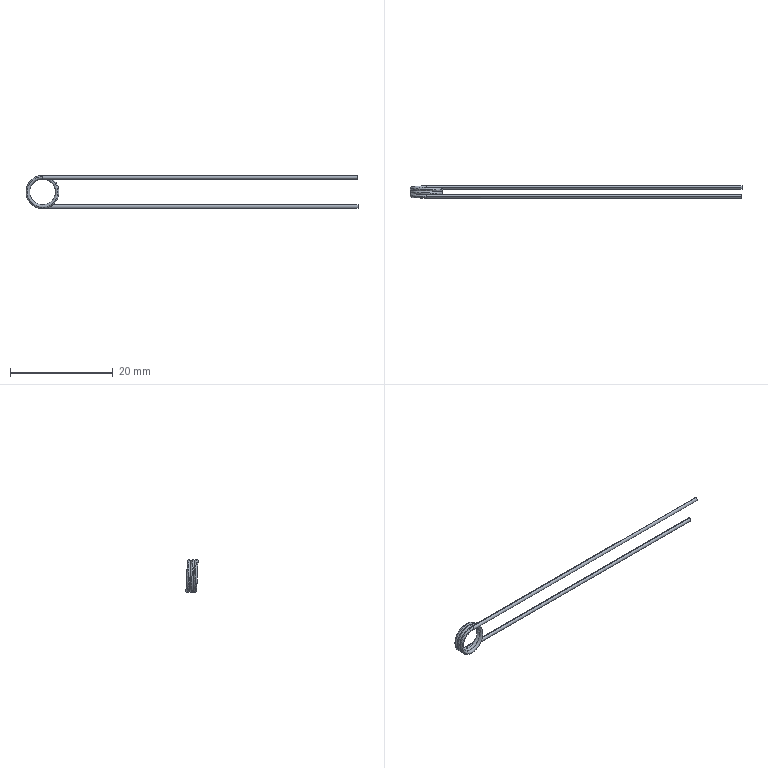Part | SolidWorks | features MoveFace 2, CompositeCurve 1, Helix 1, Sweep 1 | 1 solid | 9 faces | box 64.55 x 2.45 x 6.4 mm | volume 63.849 mm3 | cylinder 4 | spline 3 | plane 2 | commonest cylinder face diameters 0.7 x4
STEP:
#1=CARTESIAN_POINT('',(61.35,1.75,-3.2));
#2=VERTEX_POINT('',#1);
#3=CARTESIAN_POINT('',(61.35,1.75,-2.5));
#4=VERTEX_POINT('',#3);
#5=CARTESIAN_POINT('',(61.35,1.75,-2.85));
#6=DIRECTION('',(1.,0.,0.));
#7=DIRECTION('',(0.,0.00009155,-1.));
#8=AXIS2_PLACEMENT_3D('',#5,#6,#7);
#9=CIRCLE('',#8,0.35);
#10=EDGE_CURVE('',#2,#4,#9,.T.);
#11=ORIENTED_EDGE('',*,*,#10,.F.);
#12=CARTESIAN_POINT('',(-0.000000536,1.75,-3.2));
#13=VERTEX_POINT('',#12);
#14=CARTESIAN_POINT('',(12.85,1.75,-3.2));
#15=DIRECTION('',(-1.,0.,0.));
#16=VECTOR('',#15,1000.);
#17=LINE('',#14,#16);
#18=EDGE_CURVE('',#2,#13,#17,.T.);
#19=ORIENTED_EDGE('',*,*,#18,.T.);
#20=CARTESIAN_POINT('',(-0.006305,2.074,-2.979));
#21=VERTEX_POINT('',#20);
#22=CARTESIAN_POINT('',(0.,1.75,-2.85));
#23=DIRECTION('',(1.,0.,0.));
#24=DIRECTION('',(0.,0.00009155,-1.));
#25=AXIS2_PLACEMENT_3D('',#22,#23,#24);
#26=CIRCLE('',#25,0.35);
#27=EDGE_CURVE('',#13,#21,#26,.T.);
#28=ORIENTED_EDGE('',*,*,#27,.T.);
#29=CARTESIAN_POINT('',(0.,1.75,-2.5));
#30=VERTEX_POINT('',#29);
#31=CARTESIAN_POINT('',(0.,1.75,-2.85));
#32=DIRECTION('',(1.,0.,0.));
#33=DIRECTION('',(0.,0.00009155,-1.));
#34=AXIS2_PLACEMENT_3D('',#31,#32,#33);
#35=CIRCLE('',#34,0.35);
#36=EDGE_CURVE('',#21,#30,#35,.T.);
#37=ORIENTED_EDGE('',*,*,#36,.T.);
#38=CARTESIAN_POINT('',(12.85,1.75,-2.5));
#39=DIRECTION('',(-1.,0.,0.));
#40=VECTOR('',#39,1000.);
#41=LINE('',#38,#40);
#42=EDGE_CURVE('',#4,#30,#41,.T.);
#43=ORIENTED_EDGE('',*,*,#42,.F.);
#44=EDGE_LOOP('',(#11,#19,#28,#37,#43));
#45=FACE_OUTER_BOUND('',#44,.T.);
#46=CARTESIAN_POINT('',(12.85,1.75,-2.85));
#47=DIRECTION('',(-1.,0.,0.));
#48=DIRECTION('',(0.,0.,1.));
#49=AXIS2_PLACEMENT_3D('',#46,#47,#48);
#50=CYLINDRICAL_SURFACE('',#49,0.35);
#51=ADVANCED_FACE('',(#45),#50,.T.);
#52=CARTESIAN_POINT('',(0.006305,0.3239,2.979));
#53=VERTEX_POINT('',#52);
#54=CARTESIAN_POINT('',(0.,0.,3.2));
#55=VERTEX_POINT('',#54);
#56=CARTESIAN_POINT('',(0.006305,0.3239,2.979));
#57=CARTESIAN_POINT('',(0.01048,0.2681,3.104));
#58=CARTESIAN_POINT('',(0.005425,0.1388,3.2));
#59=CARTESIAN_POINT('',(0.,0.,3.2));
#60=B_SPLINE_CURVE_WITH_KNOTS('',3,(#56,#57,#58,#59),.UNSPECIFIED.,.F.,.F.,(4,4),(0.00002721,0.1895),.UNSPECIFIED.);
#61=EDGE_CURVE('',#53,#55,#60,.T.);
#62=ORIENTED_EDGE('',*,*,#61,.T.);
#63=CARTESIAN_POINT('',(61.35,0.,3.2));
#64=VERTEX_POINT('',#63);
#65=CARTESIAN_POINT('',(0.,0.,3.2));
#66=DIRECTION('',(1.,0.,0.));
#67=VECTOR('',#66,1000.);
#68=LINE('',#65,#67);
#69=EDGE_CURVE('',#55,#64,#68,.T.);
#70=ORIENTED_EDGE('',*,*,#69,.T.);
#71=CARTESIAN_POINT('',(61.35,0.,2.5));
#72=VERTEX_POINT('',#71);
#73=CARTESIAN_POINT('',(61.35,0.,2.85));
#74=DIRECTION('',(-1.,0.,0.));
#75=DIRECTION('',(0.,0.,1.));
#76=AXIS2_PLACEMENT_3D('',#73,#74,#75);
#77=CIRCLE('',#76,0.35);
#78=EDGE_CURVE('',#64,#72,#77,.T.);
#79=ORIENTED_EDGE('',*,*,#78,.T.);
#80=CARTESIAN_POINT('',(0.,0.,2.5));
#81=VERTEX_POINT('',#80);
#82=CARTESIAN_POINT('',(0.,0.,2.5));
#83=DIRECTION('',(1.,0.,0.));
#84=VECTOR('',#83,1000.);
#85=LINE('',#82,#84);
#86=EDGE_CURVE('',#81,#72,#85,.T.);
#87=ORIENTED_EDGE('',*,*,#86,.F.);
#88=CARTESIAN_POINT('',(0.,0.,2.85));
#89=DIRECTION('',(-1.,0.,0.));
#90=DIRECTION('',(0.,0.,1.));
#91=AXIS2_PLACEMENT_3D('',#88,#89,#90);
#92=CIRCLE('',#91,0.35);
#93=EDGE_CURVE('',#53,#81,#92,.T.);
#94=ORIENTED_EDGE('',*,*,#93,.F.);
#95=EDGE_LOOP('',(#62,#70,#79,#87,#94));
#96=FACE_OUTER_BOUND('',#95,.T.);
#97=CARTESIAN_POINT('',(0.,0.,2.85));
#98=DIRECTION('',(1.,0.,0.));
#99=DIRECTION('',(0.,0.,-1.));
#100=AXIS2_PLACEMENT_3D('',#97,#98,#99);
#101=CYLINDRICAL_SURFACE('',#100,0.35);
#102=ADVANCED_FACE('',(#96),#101,.T.);
#103=ORIENTED_EDGE('',*,*,#18,.F.);
#104=CARTESIAN_POINT('',(61.35,1.75,-2.85));
#105=DIRECTION('',(1.,0.,0.));
#106=DIRECTION('',(0.,0.00009155,-1.));
#107=AXIS2_PLACEMENT_3D('',#104,#105,#106);
#108=CIRCLE('',#107,0.35);
#109=EDGE_CURVE('',#4,#2,#108,.T.);
#110=ORIENTED_EDGE('',*,*,#109,.F.);
#111=ORIENTED_EDGE('',*,*,#42,.T.);
#112=CARTESIAN_POINT('',(0.006304,1.426,-2.979));
#113=VERTEX_POINT('',#112);
#114=CARTESIAN_POINT('',(0.,1.75,-2.85));
#115=DIRECTION('',(1.,0.,0.));
#116=DIRECTION('',(0.,0.00009155,-1.));
#117=AXIS2_PLACEMENT_3D('',#114,#115,#116);
#118=CIRCLE('',#117,0.35);
#119=EDGE_CURVE('',#30,#113,#118,.T.);
#120=ORIENTED_EDGE('',*,*,#119,.T.);
#121=CARTESIAN_POINT('',(0.,1.75,-2.85));
#122=DIRECTION('',(1.,0.,0.));
#123=DIRECTION('',(0.,0.00009155,-1.));
#124=AXIS2_PLACEMENT_3D('',#121,#122,#123);
#125=CIRCLE('',#124,0.35);
#126=EDGE_CURVE('',#113,#13,#125,.T.);
#127=ORIENTED_EDGE('',*,*,#126,.T.);
#128=EDGE_LOOP('',(#103,#110,#111,#120,#127));
#129=FACE_OUTER_BOUND('',#128,.T.);
#130=CARTESIAN_POINT('',(12.85,1.75,-2.85));
#131=DIRECTION('',(-1.,0.,0.));
#132=DIRECTION('',(0.,0.,1.));
#133=AXIS2_PLACEMENT_3D('',#130,#131,#132);
#134=CYLINDRICAL_SURFACE('',#133,0.35);
#135=ADVANCED_FACE('',(#129),#134,.T.);
#136=ORIENTED_EDGE('',*,*,#36,.F.);
#137=CARTESIAN_POINT('',(0.006305,0.3239,2.979));
#138=CARTESIAN_POINT('',(-0.7712,0.3519,2.981));
#139=CARTESIAN_POINT('',(-1.545,0.381,2.663));
#140=CARTESIAN_POINT('',(-2.649,0.4392,1.566));
#141=CARTESIAN_POINT('',(-2.975,0.4683,0.7939));
#142=CARTESIAN_POINT('',(-2.98,0.5195,-0.5733));
#143=CARTESIAN_POINT('',(-2.806,0.5413,-1.156));
#144=CARTESIAN_POINT('',(-2.162,0.585,-2.13));
#145=CARTESIAN_POINT('',(-1.69,0.6069,-2.521));
#146=CARTESIAN_POINT('',(-0.4324,0.658,-3.048));
#147=CARTESIAN_POINT('',(0.405,0.6871,-3.052));
#148=CARTESIAN_POINT('',(1.67,0.7383,-2.534));
#149=CARTESIAN_POINT('',(2.142,0.7601,-2.15));
#150=CARTESIAN_POINT('',(2.795,0.8037,-1.182));
#151=CARTESIAN_POINT('',(2.976,0.8257,-0.5972));
#152=CARTESIAN_POINT('',(2.981,0.8768,0.7668));
#153=CARTESIAN_POINT('',(2.665,0.9058,1.542));
#154=CARTESIAN_POINT('',(1.702,0.957,2.513));
#155=CARTESIAN_POINT('',(1.167,0.9788,2.801));
#156=CARTESIAN_POINT('',(0.02248,1.022,3.035));
#157=CARTESIAN_POINT('',(-0.587,1.044,2.978));
#158=CARTESIAN_POINT('',(-1.849,1.096,2.461));
#159=CARTESIAN_POINT('',(-2.445,1.125,1.872));
#160=CARTESIAN_POINT('',(-2.973,1.176,0.6109));
#161=CARTESIAN_POINT('',(-3.035,1.198,0.005944));
#162=CARTESIAN_POINT('',(-2.812,1.241,-1.14));
#163=CARTESIAN_POINT('',(-2.526,1.263,-1.682));
#164=CARTESIAN_POINT('',(-1.566,1.314,-2.65));
#165=CARTESIAN_POINT('',(-0.7938,1.343,-2.975));
#166=CARTESIAN_POINT('',(0.5733,1.395,-2.98));
#167=CARTESIAN_POINT('',(1.156,1.416,-2.806));
#168=CARTESIAN_POINT('',(2.13,1.46,-2.162));
#169=CARTESIAN_POINT('',(2.521,1.482,-1.69));
#170=CARTESIAN_POINT('',(3.048,1.533,-0.4324));
#171=CARTESIAN_POINT('',(3.052,1.562,0.405));
#172=CARTESIAN_POINT('',(2.534,1.613,1.67));
#173=CARTESIAN_POINT('',(2.15,1.635,2.142));
#174=CARTESIAN_POINT('',(1.182,1.679,2.795));
#175=CARTESIAN_POINT('',(0.5972,1.701,2.976));
#176=CARTESIAN_POINT('',(-0.7668,1.752,2.981));
#177=CARTESIAN_POINT('',(-1.542,1.781,2.665));
#178=CARTESIAN_POINT('',(-2.513,1.832,1.702));
#179=CARTESIAN_POINT('',(-2.801,1.854,1.167));
#180=CARTESIAN_POINT('',(-3.034,1.897,0.0225));
#181=CARTESIAN_POINT('',(-2.978,1.919,-0.587));
#182=CARTESIAN_POINT('',(-2.46,1.971,-1.85));
#183=CARTESIAN_POINT('',(-1.872,2.,-2.445));
#184=CARTESIAN_POINT('',(-0.7917,2.043,-2.897));
#185=CARTESIAN_POINT('',(-0.4042,2.058,-2.976));
#186=CARTESIAN_POINT('',(-0.006305,2.074,-2.979));
#187=B_SPLINE_CURVE_WITH_KNOTS('',3,(#137,#138,#139,#140,#141,#142,#143,#144,#145,#146,#147,#148,#149,#150,#151,#152,#153,#154,#155,#156,#157,#158,#159,#160,#161,#162,#163,#164,#165,#166,#167,#168,#169,#170,#171,#172,#173,#174,#175,#176,#177,#178,#179,#180,#181,#182,#183,#184,#185,#186),.UNSPECIFIED.,.F.,.F.,(4,2,2,2,2,2,2,2,2,2,2,2,2,2,2,2,2,2,2,2,2,2,2,2,4),(0.,0.04998,0.09999,0.1375,0.175,0.225,0.2625,0.3,0.35,0.3875,0.425,0.475,0.5125,0.55,0.6,0.6375,0.675,0.725,0.7625,0.8,0.85,0.8875,0.925,0.975,1.),.UNSPECIFIED.);
#188=EDGE_CURVE('',#53,#21,#187,.T.);
#189=ORIENTED_EDGE('',*,*,#188,.F.);
#190=ORIENTED_EDGE('',*,*,#93,.T.);
#191=CARTESIAN_POINT('',(-0.006304,-0.3239,2.979));
#192=VERTEX_POINT('',#191);
#193=CARTESIAN_POINT('',(0.,0.,2.85));
#194=DIRECTION('',(-1.,0.,0.));
#195=DIRECTION('',(0.,0.,1.));
#196=AXIS2_PLACEMENT_3D('',#193,#194,#195);
#197=CIRCLE('',#196,0.35);
#198=EDGE_CURVE('',#81,#192,#197,.T.);
#199=ORIENTED_EDGE('',*,*,#198,.T.);
#200=CARTESIAN_POINT('',(0.006304,1.426,-2.979));
#201=CARTESIAN_POINT('',(-0.379,1.413,-2.98));
#202=CARTESIAN_POINT('',(-0.7673,1.398,-2.904));
#203=CARTESIAN_POINT('',(-1.851,1.354,-2.461));
#204=CARTESIAN_POINT('',(-2.445,1.325,-1.871));
#205=CARTESIAN_POINT('',(-2.973,1.274,-0.6122));
#206=CARTESIAN_POINT('',(-3.035,1.252,-0.003211));
#207=CARTESIAN_POINT('',(-2.811,1.209,1.143));
#208=CARTESIAN_POINT('',(-2.527,1.187,1.681));
#209=CARTESIAN_POINT('',(-1.565,1.136,2.652));
#210=CARTESIAN_POINT('',(-0.792,1.107,2.975));
#211=CARTESIAN_POINT('',(0.572,1.056,2.981));
#212=CARTESIAN_POINT('',(1.158,1.034,2.805));
#213=CARTESIAN_POINT('',(2.132,0.99,2.16));
#214=CARTESIAN_POINT('',(2.52,0.9682,1.692));
#215=CARTESIAN_POINT('',(3.049,0.917,0.4308));
#216=CARTESIAN_POINT('',(3.052,0.8879,-0.4067));
#217=CARTESIAN_POINT('',(2.535,0.8368,-1.669));
#218=CARTESIAN_POINT('',(2.148,0.8149,-2.144));
#219=CARTESIAN_POINT('',(1.18,0.7712,-2.796));
#220=CARTESIAN_POINT('',(0.5985,0.7494,-2.976));
#221=CARTESIAN_POINT('',(-0.7686,0.6982,-2.981));
#222=CARTESIAN_POINT('',(-1.544,0.6692,-2.664));
#223=CARTESIAN_POINT('',(-2.512,0.6181,-1.703));
#224=CARTESIAN_POINT('',(-2.802,0.5961,-1.164));
#225=CARTESIAN_POINT('',(-3.035,0.5525,-0.01977));
#226=CARTESIAN_POINT('',(-2.978,0.5307,0.5858));
#227=CARTESIAN_POINT('',(-2.46,0.4795,1.851));
#228=CARTESIAN_POINT('',(-1.87,0.4504,2.445));
#229=CARTESIAN_POINT('',(-0.6122,0.3993,2.973));
#230=CARTESIAN_POINT('',(-0.003226,0.3774,3.035));
#231=CARTESIAN_POINT('',(1.143,0.3337,2.811));
#232=CARTESIAN_POINT('',(1.681,0.3119,2.527));
#233=CARTESIAN_POINT('',(2.652,0.2607,1.565));
#234=CARTESIAN_POINT('',(2.975,0.2317,0.792));
#235=CARTESIAN_POINT('',(2.981,0.1806,-0.572));
#236=CARTESIAN_POINT('',(2.805,0.1586,-1.158));
#237=CARTESIAN_POINT('',(2.16,0.115,-2.132));
#238=CARTESIAN_POINT('',(1.692,0.09317,-2.52));
#239=CARTESIAN_POINT('',(0.4308,0.04196,-3.049));
#240=CARTESIAN_POINT('',(-0.4067,0.01292,-3.052));
#241=CARTESIAN_POINT('',(-1.669,-0.03818,-2.535));
#242=CARTESIAN_POINT('',(-2.144,-0.06013,-2.148));
#243=CARTESIAN_POINT('',(-2.796,-0.1038,-1.18));
#244=CARTESIAN_POINT('',(-2.976,-0.1256,-0.5985));
#245=CARTESIAN_POINT('',(-2.981,-0.1768,0.7687));
#246=CARTESIAN_POINT('',(-2.663,-0.2059,1.544));
#247=CARTESIAN_POINT('',(-1.567,-0.2642,2.65));
#248=CARTESIAN_POINT('',(-0.7966,-0.2932,2.975));
#249=CARTESIAN_POINT('',(-0.006304,-0.3239,2.979));
#250=B_SPLINE_CURVE_WITH_KNOTS('',3,(#200,#201,#202,#203,#204,#205,#206,#207,#208,#209,#210,#211,#212,#213,#214,#215,#216,#217,#218,#219,#220,#221,#222,#223,#224,#225,#226,#227,#228,#229,#230,#231,#232,#233,#234,#235,#236,#237,#238,#239,#240,#241,#242,#243,#244,#245,#246,#247,#248,#249),.UNSPECIFIED.,.F.,.F.,(4,2,2,2,2,2,2,2,2,2,2,2,2,2,2,2,2,2,2,2,2,2,2,2,4),(0.,0.02496,0.07501,0.1125,0.15,0.2,0.2375,0.275,0.325,0.3625,0.4,0.45,0.4875,0.525,0.575,0.6125,0.65,0.7,0.7375,0.775,0.825,0.8625,0.9,0.95,1.),.UNSPECIFIED.);
#251=EDGE_CURVE('',#113,#192,#250,.T.);
#252=ORIENTED_EDGE('',*,*,#251,.F.);
#253=ORIENTED_EDGE('',*,*,#119,.F.);
#254=EDGE_LOOP('',(#136,#189,#190,#199,#252,#253));
#255=FACE_OUTER_BOUND('',#254,.T.);
#256=CARTESIAN_POINT('',(-0.01261,2.073,-2.978));
#257=CARTESIAN_POINT('',(-0.9931,2.036,-2.974));
#258=CARTESIAN_POINT('',(-1.942,2.,-2.452));
#259=CARTESIAN_POINT('',(-3.022,1.927,-0.8338));
#260=CARTESIAN_POINT('',(-3.123,1.89,0.2539));
#261=CARTESIAN_POINT('',(-2.369,1.817,2.048));
#262=CARTESIAN_POINT('',(-1.523,1.781,2.732));
#263=CARTESIAN_POINT('',(0.3864,1.708,3.111));
#264=CARTESIAN_POINT('',(1.43,1.671,2.788));
#265=CARTESIAN_POINT('',(2.798,1.599,1.405));
#266=CARTESIAN_POINT('',(3.107,1.562,0.3615));
#267=CARTESIAN_POINT('',(2.726,1.489,-1.547));
#268=CARTESIAN_POINT('',(2.029,1.453,-2.388));
#269=CARTESIAN_POINT('',(0.2273,1.38,-3.123));
#270=CARTESIAN_POINT('',(-0.8551,1.343,-3.009));
#271=CARTESIAN_POINT('',(-2.473,1.271,-1.927));
#272=CARTESIAN_POINT('',(-2.982,1.234,-0.9604));
#273=CARTESIAN_POINT('',(-2.972,1.161,0.9852));
#274=CARTESIAN_POINT('',(-2.453,1.125,1.942));
#275=CARTESIAN_POINT('',(-0.8335,1.052,3.022));
#276=CARTESIAN_POINT('',(0.2539,1.015,3.123));
#277=CARTESIAN_POINT('',(2.048,0.9425,2.369));
#278=CARTESIAN_POINT('',(2.732,0.9059,1.523));
#279=CARTESIAN_POINT('',(3.111,0.8331,-0.3864));
#280=CARTESIAN_POINT('',(2.788,0.7965,-1.43));
#281=CARTESIAN_POINT('',(1.405,0.7237,-2.798));
#282=CARTESIAN_POINT('',(0.3615,0.6872,-3.107));
#283=CARTESIAN_POINT('',(-1.547,0.6143,-2.726));
#284=CARTESIAN_POINT('',(-2.388,0.5777,-2.029));
#285=CARTESIAN_POINT('',(-3.123,0.505,-0.2273));
#286=CARTESIAN_POINT('',(-3.009,0.4684,0.8554));
#287=CARTESIAN_POINT('',(-1.927,0.3956,2.473));
#288=CARTESIAN_POINT('',(-0.9676,0.3593,2.982));
#289=CARTESIAN_POINT('',(0.01261,0.3226,2.978));
#290=CARTESIAN_POINT('',(-0.0161,2.162,-2.771));
#291=CARTESIAN_POINT('',(-0.9269,2.125,-2.766));
#292=CARTESIAN_POINT('',(-1.811,2.089,-2.279));
#293=CARTESIAN_POINT('',(-2.813,2.016,-0.7712));
#294=CARTESIAN_POINT('',(-2.906,1.979,0.2409));
#295=CARTESIAN_POINT('',(-2.201,1.907,1.909));
#296=CARTESIAN_POINT('',(-1.413,1.87,2.545));
#297=CARTESIAN_POINT('',(0.3644,1.797,2.894));
#298=CARTESIAN_POINT('',(1.334,1.761,2.592));
#299=CARTESIAN_POINT('',(2.606,1.688,1.303));
#300=CARTESIAN_POINT('',(2.892,1.651,0.3318));
#301=CARTESIAN_POINT('',(2.535,1.579,-1.444));
#302=CARTESIAN_POINT('',(1.884,1.542,-2.225));
#303=CARTESIAN_POINT('',(0.2064,1.469,-2.907));
#304=CARTESIAN_POINT('',(-0.8001,1.433,-2.799));
#305=CARTESIAN_POINT('',(-2.304,1.36,-1.789));
#306=CARTESIAN_POINT('',(-2.777,1.323,-0.8894));
#307=CARTESIAN_POINT('',(-2.764,1.25,0.9216));
#308=CARTESIAN_POINT('',(-2.279,1.214,1.81));
#309=CARTESIAN_POINT('',(-0.771,1.141,2.814));
#310=CARTESIAN_POINT('',(0.2409,1.104,2.906));
#311=CARTESIAN_POINT('',(1.909,1.032,2.201));
#312=CARTESIAN_POINT('',(2.545,0.9951,1.413));
#313=CARTESIAN_POINT('',(2.894,0.9223,-0.3644));
#314=CARTESIAN_POINT('',(2.592,0.8857,-1.334));
#315=CARTESIAN_POINT('',(1.303,0.8129,-2.606));
#316=CARTESIAN_POINT('',(0.3318,0.7764,-2.892));
#317=CARTESIAN_POINT('',(-1.444,0.7035,-2.535));
#318=CARTESIAN_POINT('',(-2.225,0.667,-1.884));
#319=CARTESIAN_POINT('',(-2.907,0.5942,-0.2064));
#320=CARTESIAN_POINT('',(-2.798,0.5576,0.8003));
#321=CARTESIAN_POINT('',(-1.789,0.4848,2.304));
#322=CARTESIAN_POINT('',(-0.8958,0.4485,2.776));
#323=CARTESIAN_POINT('',(0.0161,0.4118,2.771));
#324=CARTESIAN_POINT('',(-0.008888,1.977,-2.5));
#325=CARTESIAN_POINT('',(-0.8283,1.941,-2.497));
#326=CARTESIAN_POINT('',(-1.629,1.904,-2.059));
#327=CARTESIAN_POINT('',(-2.536,1.832,-0.7012));
#328=CARTESIAN_POINT('',(-2.622,1.795,0.2114));
#329=CARTESIAN_POINT('',(-1.989,1.722,1.718));
#330=CARTESIAN_POINT('',(-1.28,1.686,2.292));
#331=CARTESIAN_POINT('',(0.3232,1.613,2.612));
#332=CARTESIAN_POINT('',(1.199,1.576,2.341));
#333=CARTESIAN_POINT('',(2.349,1.503,1.18));
#334=CARTESIAN_POINT('',(2.608,1.467,0.3051));
#335=CARTESIAN_POINT('',(2.29,1.394,-1.298));
#336=CARTESIAN_POINT('',(1.704,1.358,-2.003));
#337=CARTESIAN_POINT('',(0.1914,1.285,-2.622));
#338=CARTESIAN_POINT('',(-0.716,1.248,-2.526));
#339=CARTESIAN_POINT('',(-2.075,1.175,-1.618));
#340=CARTESIAN_POINT('',(-2.503,1.139,-0.808));
#341=CARTESIAN_POINT('',(-2.495,1.066,0.8264));
#342=CARTESIAN_POINT('',(-2.06,1.029,1.628));
#343=CARTESIAN_POINT('',(-0.701,0.9565,2.537));
#344=CARTESIAN_POINT('',(0.2114,0.92,2.622));
#345=CARTESIAN_POINT('',(1.718,0.8471,1.989));
#346=CARTESIAN_POINT('',(2.292,0.8107,1.28));
#347=CARTESIAN_POINT('',(2.612,0.7378,-0.3232));
#348=CARTESIAN_POINT('',(2.341,0.7013,-1.199));
#349=CARTESIAN_POINT('',(1.18,0.6284,-2.349));
#350=CARTESIAN_POINT('',(0.3051,0.5919,-2.608));
#351=CARTESIAN_POINT('',(-1.298,0.519,-2.29));
#352=CARTESIAN_POINT('',(-2.003,0.4825,-1.704));
#353=CARTESIAN_POINT('',(-2.622,0.4096,-0.1914));
#354=CARTESIAN_POINT('',(-2.525,0.3732,0.7162));
#355=CARTESIAN_POINT('',(-1.619,0.3003,2.075));
#356=CARTESIAN_POINT('',(-0.8134,0.2639,2.503));
#357=CARTESIAN_POINT('',(0.008889,0.2274,2.5));
#358=CARTESIAN_POINT('',(0.008895,1.522,-2.5));
#359=CARTESIAN_POINT('',(-0.8105,1.486,-2.503));
#360=CARTESIAN_POINT('',(-1.614,1.45,-2.071));
#361=CARTESIAN_POINT('',(-2.532,1.377,-0.7193));
#362=CARTESIAN_POINT('',(-2.623,1.34,0.1927));
#363=CARTESIAN_POINT('',(-2.001,1.267,1.704));
#364=CARTESIAN_POINT('',(-1.296,1.231,2.283));
#365=CARTESIAN_POINT('',(0.3046,1.158,2.614));
#366=CARTESIAN_POINT('',(1.182,1.121,2.35));
#367=CARTESIAN_POINT('',(2.341,1.048,1.197));
#368=CARTESIAN_POINT('',(2.606,1.012,0.3236));
#369=CARTESIAN_POINT('',(2.299,0.9391,-1.282));
#370=CARTESIAN_POINT('',(1.719,0.9026,-1.991));
#371=CARTESIAN_POINT('',(0.2101,0.8297,-2.62));
#372=CARTESIAN_POINT('',(-0.6981,0.7933,-2.531));
#373=CARTESIAN_POINT('',(-2.064,0.7204,-1.633));
#374=CARTESIAN_POINT('',(-2.497,0.6839,-0.8259));
#375=CARTESIAN_POINT('',(-2.501,0.611,0.8087));
#376=CARTESIAN_POINT('',(-2.071,0.5745,1.614));
#377=CARTESIAN_POINT('',(-0.7191,0.5016,2.532));
#378=CARTESIAN_POINT('',(0.1927,0.4651,2.623));
#379=CARTESIAN_POINT('',(1.704,0.3922,2.001));
#380=CARTESIAN_POINT('',(2.283,0.3558,1.296));
#381=CARTESIAN_POINT('',(2.614,0.2829,-0.3046));
#382=CARTESIAN_POINT('',(2.35,0.2464,-1.182));
#383=CARTESIAN_POINT('',(1.197,0.1735,-2.341));
#384=CARTESIAN_POINT('',(0.3236,0.137,-2.606));
#385=CARTESIAN_POINT('',(-1.282,0.0641,-2.299));
#386=CARTESIAN_POINT('',(-1.991,0.02763,-1.719));
#387=CARTESIAN_POINT('',(-2.62,-0.04528,-0.2101));
#388=CARTESIAN_POINT('',(-2.531,-0.08173,0.6983));
#389=CARTESIAN_POINT('',(-1.633,-0.1546,2.064));
#390=CARTESIAN_POINT('',(-0.8313,-0.191,2.497));
#391=CARTESIAN_POINT('',(-0.008894,-0.2275,2.5));
#392=CARTESIAN_POINT('',(0.0161,1.338,-2.771));
#393=CARTESIAN_POINT('',(-0.8947,1.302,-2.777));
#394=CARTESIAN_POINT('',(-1.785,1.265,-2.3));
#395=CARTESIAN_POINT('',(-2.804,1.192,-0.804));
#396=CARTESIAN_POINT('',(-2.908,1.156,0.2071));
#397=CARTESIAN_POINT('',(-2.223,1.083,1.884));
#398=CARTESIAN_POINT('',(-1.443,1.046,2.528));
#399=CARTESIAN_POINT('',(0.3307,0.9736,2.899));
#400=CARTESIAN_POINT('',(1.304,0.937,2.608));
#401=CARTESIAN_POINT('',(2.591,0.8642,1.333));
#402=CARTESIAN_POINT('',(2.888,0.8277,0.3653));
#403=CARTESIAN_POINT('',(2.552,0.7548,-1.415));
#404=CARTESIAN_POINT('',(1.91,0.7183,-2.203));
#405=CARTESIAN_POINT('',(0.2402,0.6455,-2.904));
#406=CARTESIAN_POINT('',(-0.7677,0.6089,-2.808));
#407=CARTESIAN_POINT('',(-2.284,0.5361,-1.816));
#408=CARTESIAN_POINT('',(-2.766,0.4995,-0.9217));
#409=CARTESIAN_POINT('',(-2.775,0.4267,0.8895));
#410=CARTESIAN_POINT('',(-2.3,0.3902,1.784));
#411=CARTESIAN_POINT('',(-0.8038,0.3173,2.805));
#412=CARTESIAN_POINT('',(0.2071,0.2808,2.908));
#413=CARTESIAN_POINT('',(1.884,0.208,2.223));
#414=CARTESIAN_POINT('',(2.528,0.1714,1.443));
#415=CARTESIAN_POINT('',(2.899,0.09857,-0.3307));
#416=CARTESIAN_POINT('',(2.608,0.06204,-1.304));
#417=CARTESIAN_POINT('',(1.333,-0.01079,-2.591));
#418=CARTESIAN_POINT('',(0.3653,-0.0473,-2.888));
#419=CARTESIAN_POINT('',(-1.415,-0.1202,-2.552));
#420=CARTESIAN_POINT('',(-2.203,-0.1567,-1.91));
#421=CARTESIAN_POINT('',(-2.904,-0.2295,-0.2402));
#422=CARTESIAN_POINT('',(-2.807,-0.2661,0.7679));
#423=CARTESIAN_POINT('',(-1.816,-0.3389,2.283));
#424=CARTESIAN_POINT('',(-0.9282,-0.3752,2.766));
#425=CARTESIAN_POINT('',(-0.0161,-0.4119,2.771));
#426=CARTESIAN_POINT('',(0.01261,1.427,-2.978));
#427=CARTESIAN_POINT('',(-0.9679,1.391,-2.982));
#428=CARTESIAN_POINT('',(-1.922,1.354,-2.469));
#429=CARTESIAN_POINT('',(-3.015,1.282,-0.8595));
#430=CARTESIAN_POINT('',(-3.125,1.245,0.2275));
#431=CARTESIAN_POINT('',(-2.386,1.172,2.028));
#432=CARTESIAN_POINT('',(-1.546,1.136,2.72));
#433=CARTESIAN_POINT('',(0.36,1.063,3.114));
#434=CARTESIAN_POINT('',(1.406,1.026,2.8));
#435=CARTESIAN_POINT('',(2.787,0.9536,1.429));
#436=CARTESIAN_POINT('',(3.104,0.917,0.3878));
#437=CARTESIAN_POINT('',(2.739,0.8442,-1.524));
#438=CARTESIAN_POINT('',(2.049,0.8076,-2.37));
#439=CARTESIAN_POINT('',(0.2537,0.7349,-3.121));
#440=CARTESIAN_POINT('',(-0.8297,0.6983,-3.016));
#441=CARTESIAN_POINT('',(-2.457,0.6254,-1.948));
#442=CARTESIAN_POINT('',(-2.974,0.5889,-0.9857));
#443=CARTESIAN_POINT('',(-2.981,0.5161,0.96));
#444=CARTESIAN_POINT('',(-2.469,0.4795,1.921));
#445=CARTESIAN_POINT('',(-0.8592,0.4067,3.015));
#446=CARTESIAN_POINT('',(0.2275,0.3701,3.125));
#447=CARTESIAN_POINT('',(2.028,0.2974,2.386));
#448=CARTESIAN_POINT('',(2.72,0.2608,1.546));
#449=CARTESIAN_POINT('',(3.114,0.1879,-0.36));
#450=CARTESIAN_POINT('',(2.8,0.1514,-1.406));
#451=CARTESIAN_POINT('',(1.429,0.07861,-2.787));
#452=CARTESIAN_POINT('',(0.3878,0.04204,-3.104));
#453=CARTESIAN_POINT('',(-1.524,-0.03081,-2.739));
#454=CARTESIAN_POINT('',(-2.371,-0.06738,-2.049));
#455=CARTESIAN_POINT('',(-3.121,-0.1401,-0.2537));
#456=CARTESIAN_POINT('',(-3.016,-0.1767,0.83));
#457=CARTESIAN_POINT('',(-1.948,-0.2496,2.456));
#458=CARTESIAN_POINT('',(-0.993,-0.2858,2.974));
#459=CARTESIAN_POINT('',(-0.01261,-0.3225,2.978));
#460=B_SPLINE_SURFACE_WITH_KNOTS('',3,3,((#256,#257,#258,#259,#260,#261,#262,#263,#264,#265,#266,#267,#268,#269,#270,#271,#272,#273,#274,#275,#276,#277,#278,#279,#280,#281,#282,#283,#284,#285,#286,#287,#288,#289),(#290,#291,#292,#293,#294,#295,#296,#297,#298,#299,#300,#301,#302,#303,#304,#305,#306,#307,#308,#309,#310,#311,#312,#313,#314,#315,#316,#317,#318,#319,#320,#321,#322,#323),(#324,#325,#326,#327,#328,#329,#330,#331,#332,#333,#334,#335,#336,#337,#338,#339,#340,#341,#342,#343,#344,#345,#346,#347,#348,#349,#350,#351,#352,#353,#354,#355,#356,#357),(#358,#359,#360,#361,#362,#363,#364,#365,#366,#367,#368,#369,#370,#371,#372,#373,#374,#375,#376,#377,#378,#379,#380,#381,#382,#383,#384,#385,#386,#387,#388,#389,#390,#391),(#392,#393,#394,#395,#396,#397,#398,#399,#400,#401,#402,#403,#404,#405,#406,#407,#408,#409,#410,#411,#412,#413,#414,#415,#416,#417,#418,#419,#420,#421,#422,#423,#424,#425),(#426,#427,#428,#429,#430,#431,#432,#433,#434,#435,#436,#437,#438,#439,#440,#441,#442,#443,#444,#445,#446,#447,#448,#449,#450,#451,#452,#453,#454,#455,#456,#457,#458,#459)),.UNSPECIFIED.,.F.,.F.,.F.,(4,2,4),(4,2,2,2,2,2,2,2,2,2,2,2,2,2,2,2,4),(0.1895,0.5,0.8106),(0.,0.0625,0.125,0.1875,0.25,0.3125,0.375,0.4375,0.5,0.5625,0.625,0.6875,0.75,0.8125,0.875,0.9375,1.),.UNSPECIFIED.);
#461=ADVANCED_FACE('',(#255),#460,.F.);
#462=ORIENTED_EDGE('',*,*,#126,.F.);
#463=ORIENTED_EDGE('',*,*,#251,.T.);
#464=CARTESIAN_POINT('',(0.,0.,3.2));
#465=CARTESIAN_POINT('',(-0.005423,-0.1387,3.2));
#466=CARTESIAN_POINT('',(-0.01048,-0.268,3.104));
#467=CARTESIAN_POINT('',(-0.006304,-0.3239,2.979));
#468=B_SPLINE_CURVE_WITH_KNOTS('',3,(#464,#465,#466,#467),.UNSPECIFIED.,.F.,.F.,(4,4),(0.8106,1.),.UNSPECIFIED.);
#469=EDGE_CURVE('',#55,#192,#468,.T.);
#470=ORIENTED_EDGE('',*,*,#469,.F.);
#471=CARTESIAN_POINT('',(-0.000000536,1.75,-3.2));
#472=CARTESIAN_POINT('',(-0.4215,1.735,-3.2));
#473=CARTESIAN_POINT('',(-0.8371,1.721,-3.117));
#474=CARTESIAN_POINT('',(-2.001,1.677,-2.635));
#475=CARTESIAN_POINT('',(-2.635,1.648,-2.));
#476=CARTESIAN_POINT('',(-3.197,1.597,-0.6438));
#477=CARTESIAN_POINT('',(-3.261,1.575,0.01064));
#478=CARTESIAN_POINT('',(-3.015,1.531,1.241));
#479=CARTESIAN_POINT('',(-2.708,1.51,1.817));
#480=CARTESIAN_POINT('',(-1.669,1.458,2.857));
#481=CARTESIAN_POINT('',(-0.8382,1.429,3.2));
#482=CARTESIAN_POINT('',(0.6287,1.378,3.2));
#483=CARTESIAN_POINT('',(1.258,1.356,3.008));
#484=CARTESIAN_POINT('',(2.3,1.313,2.311));
#485=CARTESIAN_POINT('',(2.715,1.291,1.807));
#486=CARTESIAN_POINT('',(3.278,1.239,0.4484));
#487=CARTESIAN_POINT('',(3.277,1.211,-0.4502));
#488=CARTESIAN_POINT('',(2.716,1.159,-1.805));
#489=CARTESIAN_POINT('',(2.298,1.137,-2.313));
#490=CARTESIAN_POINT('',(1.255,1.094,-3.01));
#491=CARTESIAN_POINT('',(0.6301,1.072,-3.2));
#492=CARTESIAN_POINT('',(-0.8402,1.021,-3.2));
#493=CARTESIAN_POINT('',(-1.67,0.9918,-2.855));
#494=CARTESIAN_POINT('',(-2.707,0.9406,-1.818));
#495=CARTESIAN_POINT('',(-3.017,0.9186,-1.238));
#496=CARTESIAN_POINT('',(-3.261,0.875,-0.007701));
#497=CARTESIAN_POINT('',(-3.198,0.8533,0.6424));
#498=CARTESIAN_POINT('',(-2.635,0.8019,2.001));
#499=CARTESIAN_POINT('',(-1.999,0.773,2.636));
#500=CARTESIAN_POINT('',(-0.6438,0.7218,3.197));
#501=CARTESIAN_POINT('',(0.01062,0.6999,3.261));
#502=CARTESIAN_POINT('',(1.241,0.6563,3.015));
#503=CARTESIAN_POINT('',(1.817,0.6345,2.708));
#504=CARTESIAN_POINT('',(2.857,0.5832,1.669));
#505=CARTESIAN_POINT('',(3.2,0.5543,0.8382));
#506=CARTESIAN_POINT('',(3.2,0.5031,-0.6287));
#507=CARTESIAN_POINT('',(3.008,0.4811,-1.258));
#508=CARTESIAN_POINT('',(2.311,0.4375,-2.3));
#509=CARTESIAN_POINT('',(1.807,0.4158,-2.715));
#510=CARTESIAN_POINT('',(0.4484,0.3644,-3.278));
#511=CARTESIAN_POINT('',(-0.4502,0.3355,-3.277));
#512=CARTESIAN_POINT('',(-1.805,0.2843,-2.716));
#513=CARTESIAN_POINT('',(-2.313,0.2624,-2.298));
#514=CARTESIAN_POINT('',(-3.01,0.2188,-1.255));
#515=CARTESIAN_POINT('',(-3.2,0.197,-0.6301));
#516=CARTESIAN_POINT('',(-3.2,0.1457,0.8403));
#517=CARTESIAN_POINT('',(-2.854,0.1167,1.671));
#518=CARTESIAN_POINT('',(-1.671,0.05831,2.854));
#519=CARTESIAN_POINT('',(-0.8425,0.02943,3.2));
#520=CARTESIAN_POINT('',(0.,0.,3.2));
#521=B_SPLINE_CURVE_WITH_KNOTS('',3,(#471,#472,#473,#474,#475,#476,#477,#478,#479,#480,#481,#482,#483,#484,#485,#486,#487,#488,#489,#490,#491,#492,#493,#494,#495,#496,#497,#498,#499,#500,#501,#502,#503,#504,#505,#506,#507,#508,#509,#510,#511,#512,#513,#514,#515,#516,#517,#518,#519,#520),.UNSPECIFIED.,.F.,.F.,(4,2,2,2,2,2,2,2,2,2,2,2,2,2,2,2,2,2,2,2,2,2,2,2,4),(0.,0.02496,0.07501,0.1125,0.15,0.2,0.2375,0.275,0.325,0.3625,0.4,0.45,0.4875,0.525,0.575,0.6125,0.65,0.7,0.7375,0.775,0.825,0.8625,0.9,0.95,1.),.UNSPECIFIED.);
#522=EDGE_CURVE('',#13,#55,#521,.T.);
#523=ORIENTED_EDGE('',*,*,#522,.F.);
#524=EDGE_LOOP('',(#462,#463,#470,#523));
#525=FACE_OUTER_BOUND('',#524,.T.);
#526=CARTESIAN_POINT('',(0.01261,1.427,-2.978));
#527=CARTESIAN_POINT('',(-0.379,1.413,-2.98));
#528=CARTESIAN_POINT('',(-0.7673,1.398,-2.904));
#529=CARTESIAN_POINT('',(-1.851,1.354,-2.461));
#530=CARTESIAN_POINT('',(-2.445,1.325,-1.871));
#531=CARTESIAN_POINT('',(-2.973,1.274,-0.6122));
#532=CARTESIAN_POINT('',(-3.035,1.252,-0.003211));
#533=CARTESIAN_POINT('',(-2.811,1.209,1.143));
#534=CARTESIAN_POINT('',(-2.527,1.187,1.681));
#535=CARTESIAN_POINT('',(-1.565,1.136,2.652));
#536=CARTESIAN_POINT('',(-0.792,1.107,2.975));
#537=CARTESIAN_POINT('',(0.572,1.056,2.981));
#538=CARTESIAN_POINT('',(1.158,1.034,2.805));
#539=CARTESIAN_POINT('',(2.132,0.99,2.16));
#540=CARTESIAN_POINT('',(2.52,0.9682,1.692));
#541=CARTESIAN_POINT('',(3.049,0.917,0.4308));
#542=CARTESIAN_POINT('',(3.052,0.8879,-0.4067));
#543=CARTESIAN_POINT('',(2.535,0.8368,-1.669));
#544=CARTESIAN_POINT('',(2.148,0.8149,-2.144));
#545=CARTESIAN_POINT('',(1.18,0.7712,-2.796));
#546=CARTESIAN_POINT('',(0.5985,0.7494,-2.976));
#547=CARTESIAN_POINT('',(-0.7686,0.6982,-2.981));
#548=CARTESIAN_POINT('',(-1.544,0.6692,-2.664));
#549=CARTESIAN_POINT('',(-2.512,0.6181,-1.703));
#550=CARTESIAN_POINT('',(-2.802,0.5961,-1.164));
#551=CARTESIAN_POINT('',(-3.035,0.5525,-0.01977));
#552=CARTESIAN_POINT('',(-2.978,0.5307,0.5858));
#553=CARTESIAN_POINT('',(-2.46,0.4795,1.851));
#554=CARTESIAN_POINT('',(-1.87,0.4504,2.445));
#555=CARTESIAN_POINT('',(-0.6122,0.3993,2.973));
#556=CARTESIAN_POINT('',(-0.003226,0.3774,3.035));
#557=CARTESIAN_POINT('',(1.143,0.3337,2.811));
#558=CARTESIAN_POINT('',(1.681,0.3119,2.527));
#559=CARTESIAN_POINT('',(2.652,0.2607,1.565));
#560=CARTESIAN_POINT('',(2.975,0.2317,0.792));
#561=CARTESIAN_POINT('',(2.981,0.1806,-0.572));
#562=CARTESIAN_POINT('',(2.805,0.1586,-1.158));
#563=CARTESIAN_POINT('',(2.16,0.115,-2.132));
#564=CARTESIAN_POINT('',(1.692,0.09317,-2.52));
#565=CARTESIAN_POINT('',(0.4308,0.04196,-3.049));
#566=CARTESIAN_POINT('',(-0.4067,0.01292,-3.052));
#567=CARTESIAN_POINT('',(-1.669,-0.03818,-2.535));
#568=CARTESIAN_POINT('',(-2.144,-0.06013,-2.148));
#569=CARTESIAN_POINT('',(-2.796,-0.1038,-1.18));
#570=CARTESIAN_POINT('',(-2.976,-0.1256,-0.5985));
#571=CARTESIAN_POINT('',(-2.981,-0.1768,0.7687));
#572=CARTESIAN_POINT('',(-2.663,-0.2059,1.544));
#573=CARTESIAN_POINT('',(-1.567,-0.2642,2.65));
#574=CARTESIAN_POINT('',(-0.7966,-0.2932,2.975));
#575=CARTESIAN_POINT('',(-0.01261,-0.3225,2.978));
#576=CARTESIAN_POINT('',(0.01048,1.482,-3.104));
#577=CARTESIAN_POINT('',(-0.3981,1.467,-3.106));
#578=CARTESIAN_POINT('',(-0.802,1.453,-3.026));
#579=CARTESIAN_POINT('',(-1.932,1.409,-2.563));
#580=CARTESIAN_POINT('',(-2.55,1.38,-1.948));
#581=CARTESIAN_POINT('',(-3.099,1.329,-0.6352));
#582=CARTESIAN_POINT('',(-3.163,1.307,-0.0004747));
#583=CARTESIAN_POINT('',(-2.929,1.263,1.194));
#584=CARTESIAN_POINT('',(-2.633,1.241,1.754));
#585=CARTESIAN_POINT('',(-1.628,1.19,2.766));
#586=CARTESIAN_POINT('',(-0.8233,1.161,3.102));
#587=CARTESIAN_POINT('',(0.5992,1.11,3.106));
#588=CARTESIAN_POINT('',(1.21,1.088,2.923));
#589=CARTESIAN_POINT('',(2.224,1.044,2.249));
#590=CARTESIAN_POINT('',(2.628,1.023,1.761));
#591=CARTESIAN_POINT('',(3.178,0.9714,0.4459));
#592=CARTESIAN_POINT('',(3.181,0.9425,-0.4263));
#593=CARTESIAN_POINT('',(2.641,0.8913,-1.742));
#594=CARTESIAN_POINT('',(2.237,0.8694,-2.236));
#595=CARTESIAN_POINT('',(1.227,0.8257,-2.915));
#596=CARTESIAN_POINT('',(0.6215,0.804,-3.102));
#597=CARTESIAN_POINT('',(-0.8043,0.7527,-3.107));
#598=CARTESIAN_POINT('',(-1.611,0.7237,-2.775));
#599=CARTESIAN_POINT('',(-2.62,0.6725,-1.773));
#600=CARTESIAN_POINT('',(-2.922,0.6506,-1.211));
#601=CARTESIAN_POINT('',(-3.163,0.607,-0.01804));
#602=CARTESIAN_POINT('',(-3.104,0.5852,0.613));
#603=CARTESIAN_POINT('',(-2.563,0.5339,1.932));
#604=CARTESIAN_POINT('',(-1.948,0.505,2.55));
#605=CARTESIAN_POINT('',(-0.6352,0.4538,3.099));
#606=CARTESIAN_POINT('',(-0.0004918,0.4319,3.163));
#607=CARTESIAN_POINT('',(1.194,0.3882,2.929));
#608=CARTESIAN_POINT('',(1.754,0.3665,2.633));
#609=CARTESIAN_POINT('',(2.766,0.3152,1.628));
#610=CARTESIAN_POINT('',(3.102,0.2862,0.8233));
#611=CARTESIAN_POINT('',(3.106,0.235,-0.5992));
#612=CARTESIAN_POINT('',(2.923,0.2131,-1.21));
#613=CARTESIAN_POINT('',(2.249,0.1695,-2.224));
#614=CARTESIAN_POINT('',(1.761,0.1477,-2.628));
#615=CARTESIAN_POINT('',(0.4459,0.09641,-3.178));
#616=CARTESIAN_POINT('',(-0.4263,0.06746,-3.181));
#617=CARTESIAN_POINT('',(-1.742,0.01629,-2.641));
#618=CARTESIAN_POINT('',(-2.236,-0.005646,-2.237));
#619=CARTESIAN_POINT('',(-2.915,-0.04927,-1.227));
#620=CARTESIAN_POINT('',(-3.102,-0.07105,-0.6215));
#621=CARTESIAN_POINT('',(-3.107,-0.1223,0.8044));
#622=CARTESIAN_POINT('',(-2.774,-0.1514,1.612));
#623=CARTESIAN_POINT('',(-1.631,-0.2097,2.763));
#624=CARTESIAN_POINT('',(-0.8278,-0.2386,3.102));
#625=CARTESIAN_POINT('',(-0.01048,-0.268,3.104));
#626=CARTESIAN_POINT('',(0.005423,1.611,-3.2));
#627=CARTESIAN_POINT('',(-0.416,1.597,-3.201));
#628=CARTESIAN_POINT('',(-0.8318,1.582,-3.118));
#629=CARTESIAN_POINT('',(-1.996,1.538,-2.639));
#630=CARTESIAN_POINT('',(-2.632,1.509,-2.004));
#631=CARTESIAN_POINT('',(-3.196,1.458,-0.6492));
#632=CARTESIAN_POINT('',(-3.261,1.436,0.005106));
#633=CARTESIAN_POINT('',(-3.018,1.393,1.236));
#634=CARTESIAN_POINT('',(-2.711,1.371,1.813));
#635=CARTESIAN_POINT('',(-1.673,1.319,2.854));
#636=CARTESIAN_POINT('',(-0.8436,1.291,3.199));
#637=CARTESIAN_POINT('',(0.6232,1.239,3.201));
#638=CARTESIAN_POINT('',(1.253,1.217,3.011));
#639=CARTESIAN_POINT('',(2.296,1.174,2.315));
#640=CARTESIAN_POINT('',(2.712,1.152,1.811));
#641=CARTESIAN_POINT('',(3.277,1.101,0.4539));
#642=CARTESIAN_POINT('',(3.278,1.072,-0.4446));
#643=CARTESIAN_POINT('',(2.719,1.021,-1.801));
#644=CARTESIAN_POINT('',(2.302,0.9986,-2.309));
#645=CARTESIAN_POINT('',(1.26,0.955,-3.007));
#646=CARTESIAN_POINT('',(0.6356,0.9333,-3.199));
#647=CARTESIAN_POINT('',(-0.8348,0.8819,-3.201));
#648=CARTESIAN_POINT('',(-1.665,0.853,-2.858));
#649=CARTESIAN_POINT('',(-2.704,0.8018,-1.823));
#650=CARTESIAN_POINT('',(-3.014,0.7799,-1.243));
#651=CARTESIAN_POINT('',(-3.261,0.7363,-0.01323));
#652=CARTESIAN_POINT('',(-3.199,0.7145,0.637));
#653=CARTESIAN_POINT('',(-2.638,0.6632,1.996));
#654=CARTESIAN_POINT('',(-2.003,0.6343,2.632));
#655=CARTESIAN_POINT('',(-0.6492,0.583,3.196));
#656=CARTESIAN_POINT('',(0.005088,0.5611,3.261));
#657=CARTESIAN_POINT('',(1.236,0.5175,3.018));
#658=CARTESIAN_POINT('',(1.813,0.4958,2.711));
#659=CARTESIAN_POINT('',(2.854,0.4444,1.673));
#660=CARTESIAN_POINT('',(3.199,0.4155,0.8437));
#661=CARTESIAN_POINT('',(3.201,0.3643,-0.6232));
#662=CARTESIAN_POINT('',(3.011,0.3424,-1.253));
#663=CARTESIAN_POINT('',(2.315,0.2988,-2.296));
#664=CARTESIAN_POINT('',(1.811,0.277,-2.712));
#665=CARTESIAN_POINT('',(0.4539,0.2257,-3.277));
#666=CARTESIAN_POINT('',(-0.4446,0.1968,-3.278));
#667=CARTESIAN_POINT('',(-1.801,0.1455,-2.719));
#668=CARTESIAN_POINT('',(-2.309,0.1236,-2.302));
#669=CARTESIAN_POINT('',(-3.007,0.08004,-1.26));
#670=CARTESIAN_POINT('',(-3.199,0.05826,-0.6356));
#671=CARTESIAN_POINT('',(-3.201,0.006904,0.8348));
#672=CARTESIAN_POINT('',(-2.857,-0.02205,1.666));
#673=CARTESIAN_POINT('',(-1.676,-0.08045,2.852));
#674=CARTESIAN_POINT('',(-0.848,-0.1093,3.199));
#675=CARTESIAN_POINT('',(-0.005424,-0.1388,3.2));
#676=CARTESIAN_POINT('',(-0.000001252,1.75,-3.2));
#677=CARTESIAN_POINT('',(-0.4215,1.735,-3.2));
#678=CARTESIAN_POINT('',(-0.8371,1.721,-3.117));
#679=CARTESIAN_POINT('',(-2.001,1.677,-2.635));
#680=CARTESIAN_POINT('',(-2.635,1.648,-2.));
#681=CARTESIAN_POINT('',(-3.197,1.597,-0.6438));
#682=CARTESIAN_POINT('',(-3.261,1.575,0.01064));
#683=CARTESIAN_POINT('',(-3.015,1.531,1.241));
#684=CARTESIAN_POINT('',(-2.708,1.51,1.817));
#685=CARTESIAN_POINT('',(-1.669,1.458,2.857));
#686=CARTESIAN_POINT('',(-0.8382,1.429,3.2));
#687=CARTESIAN_POINT('',(0.6287,1.378,3.2));
#688=CARTESIAN_POINT('',(1.258,1.356,3.008));
#689=CARTESIAN_POINT('',(2.3,1.313,2.311));
#690=CARTESIAN_POINT('',(2.715,1.291,1.807));
#691=CARTESIAN_POINT('',(3.278,1.239,0.4484));
#692=CARTESIAN_POINT('',(3.277,1.211,-0.4502));
#693=CARTESIAN_POINT('',(2.716,1.159,-1.805));
#694=CARTESIAN_POINT('',(2.298,1.137,-2.313));
#695=CARTESIAN_POINT('',(1.255,1.094,-3.01));
#696=CARTESIAN_POINT('',(0.6301,1.072,-3.2));
#697=CARTESIAN_POINT('',(-0.8402,1.021,-3.2));
#698=CARTESIAN_POINT('',(-1.67,0.9918,-2.855));
#699=CARTESIAN_POINT('',(-2.707,0.9406,-1.818));
#700=CARTESIAN_POINT('',(-3.017,0.9186,-1.238));
#701=CARTESIAN_POINT('',(-3.261,0.875,-0.007701));
#702=CARTESIAN_POINT('',(-3.198,0.8533,0.6424));
#703=CARTESIAN_POINT('',(-2.635,0.8019,2.001));
#704=CARTESIAN_POINT('',(-1.999,0.773,2.636));
#705=CARTESIAN_POINT('',(-0.6438,0.7218,3.197));
#706=CARTESIAN_POINT('',(0.01062,0.6999,3.261));
#707=CARTESIAN_POINT('',(1.241,0.6563,3.015));
#708=CARTESIAN_POINT('',(1.817,0.6345,2.708));
#709=CARTESIAN_POINT('',(2.857,0.5832,1.669));
#710=CARTESIAN_POINT('',(3.2,0.5543,0.8382));
#711=CARTESIAN_POINT('',(3.2,0.5031,-0.6287));
#712=CARTESIAN_POINT('',(3.008,0.4811,-1.258));
#713=CARTESIAN_POINT('',(2.311,0.4375,-2.3));
#714=CARTESIAN_POINT('',(1.807,0.4158,-2.715));
#715=CARTESIAN_POINT('',(0.4484,0.3644,-3.278));
#716=CARTESIAN_POINT('',(-0.4502,0.3355,-3.277));
#717=CARTESIAN_POINT('',(-1.805,0.2843,-2.716));
#718=CARTESIAN_POINT('',(-2.313,0.2624,-2.298));
#719=CARTESIAN_POINT('',(-3.01,0.2188,-1.255));
#720=CARTESIAN_POINT('',(-3.2,0.197,-0.6301));
#721=CARTESIAN_POINT('',(-3.2,0.1457,0.8403));
#722=CARTESIAN_POINT('',(-2.854,0.1167,1.671));
#723=CARTESIAN_POINT('',(-1.671,0.05831,2.854));
#724=CARTESIAN_POINT('',(-0.8425,0.02943,3.2));
#725=CARTESIAN_POINT('',(0.,0.,3.2));
#726=B_SPLINE_SURFACE_WITH_KNOTS('',3,3,((#526,#527,#528,#529,#530,#531,#532,#533,#534,#535,#536,#537,#538,#539,#540,#541,#542,#543,#544,#545,#546,#547,#548,#549,#550,#551,#552,#553,#554,#555,#556,#557,#558,#559,#560,#561,#562,#563,#564,#565,#566,#567,#568,#569,#570,#571,#572,#573,#574,#575),(#576,#577,#578,#579,#580,#581,#582,#583,#584,#585,#586,#587,#588,#589,#590,#591,#592,#593,#594,#595,#596,#597,#598,#599,#600,#601,#602,#603,#604,#605,#606,#607,#608,#609,#610,#611,#612,#613,#614,#615,#616,#617,#618,#619,#620,#621,#622,#623,#624,#625),(#626,#627,#628,#629,#630,#631,#632,#633,#634,#635,#636,#637,#638,#639,#640,#641,#642,#643,#644,#645,#646,#647,#648,#649,#650,#651,#652,#653,#654,#655,#656,#657,#658,#659,#660,#661,#662,#663,#664,#665,#666,#667,#668,#669,#670,#671,#672,#673,#674,#675),(#676,#677,#678,#679,#680,#681,#682,#683,#684,#685,#686,#687,#688,#689,#690,#691,#692,#693,#694,#695,#696,#697,#698,#699,#700,#701,#702,#703,#704,#705,#706,#707,#708,#709,#710,#711,#712,#713,#714,#715,#716,#717,#718,#719,#720,#721,#722,#723,#724,#725)),.UNSPECIFIED.,.F.,.F.,.F.,(4,4),(4,2,2,2,2,2,2,2,2,2,2,2,2,2,2,2,2,2,2,2,2,2,2,2,4),(0.8106,1.),(0.,0.02496,0.07501,0.1125,0.15,0.2,0.2375,0.275,0.325,0.3625,0.4,0.45,0.4875,0.525,0.575,0.6125,0.65,0.7,0.7375,0.775,0.825,0.8625,0.9,0.95,1.),.UNSPECIFIED.);
#727=ADVANCED_FACE('',(#525),#726,.F.);
#728=ORIENTED_EDGE('',*,*,#27,.F.);
#729=ORIENTED_EDGE('',*,*,#522,.T.);
#730=ORIENTED_EDGE('',*,*,#61,.F.);
#731=ORIENTED_EDGE('',*,*,#188,.T.);
#732=EDGE_LOOP('',(#728,#729,#730,#731));
#733=FACE_OUTER_BOUND('',#732,.T.);
#734=CARTESIAN_POINT('',(-0.000001252,1.75,-3.2));
#735=CARTESIAN_POINT('',(-0.4215,1.735,-3.2));
#736=CARTESIAN_POINT('',(-0.8371,1.721,-3.117));
#737=CARTESIAN_POINT('',(-2.001,1.677,-2.635));
#738=CARTESIAN_POINT('',(-2.635,1.648,-2.));
#739=CARTESIAN_POINT('',(-3.197,1.597,-0.6438));
#740=CARTESIAN_POINT('',(-3.261,1.575,0.01064));
#741=CARTESIAN_POINT('',(-3.015,1.531,1.241));
#742=CARTESIAN_POINT('',(-2.708,1.51,1.817));
#743=CARTESIAN_POINT('',(-1.669,1.458,2.857));
#744=CARTESIAN_POINT('',(-0.8382,1.429,3.2));
#745=CARTESIAN_POINT('',(0.6287,1.378,3.2));
#746=CARTESIAN_POINT('',(1.258,1.356,3.008));
#747=CARTESIAN_POINT('',(2.3,1.313,2.311));
#748=CARTESIAN_POINT('',(2.715,1.291,1.807));
#749=CARTESIAN_POINT('',(3.278,1.239,0.4484));
#750=CARTESIAN_POINT('',(3.277,1.211,-0.4502));
#751=CARTESIAN_POINT('',(2.716,1.159,-1.805));
#752=CARTESIAN_POINT('',(2.298,1.137,-2.313));
#753=CARTESIAN_POINT('',(1.255,1.094,-3.01));
#754=CARTESIAN_POINT('',(0.6301,1.072,-3.2));
#755=CARTESIAN_POINT('',(-0.8402,1.021,-3.2));
#756=CARTESIAN_POINT('',(-1.67,0.9918,-2.855));
#757=CARTESIAN_POINT('',(-2.707,0.9406,-1.818));
#758=CARTESIAN_POINT('',(-3.017,0.9186,-1.238));
#759=CARTESIAN_POINT('',(-3.261,0.875,-0.007701));
#760=CARTESIAN_POINT('',(-3.198,0.8533,0.6424));
#761=CARTESIAN_POINT('',(-2.635,0.8019,2.001));
#762=CARTESIAN_POINT('',(-1.999,0.773,2.636));
#763=CARTESIAN_POINT('',(-0.6438,0.7218,3.197));
#764=CARTESIAN_POINT('',(0.01062,0.6999,3.261));
#765=CARTESIAN_POINT('',(1.241,0.6563,3.015));
#766=CARTESIAN_POINT('',(1.817,0.6345,2.708));
#767=CARTESIAN_POINT('',(2.857,0.5832,1.669));
#768=CARTESIAN_POINT('',(3.2,0.5543,0.8382));
#769=CARTESIAN_POINT('',(3.2,0.5031,-0.6287));
#770=CARTESIAN_POINT('',(3.008,0.4811,-1.258));
#771=CARTESIAN_POINT('',(2.311,0.4375,-2.3));
#772=CARTESIAN_POINT('',(1.807,0.4158,-2.715));
#773=CARTESIAN_POINT('',(0.4484,0.3644,-3.278));
#774=CARTESIAN_POINT('',(-0.4502,0.3355,-3.277));
#775=CARTESIAN_POINT('',(-1.805,0.2843,-2.716));
#776=CARTESIAN_POINT('',(-2.313,0.2624,-2.298));
#777=CARTESIAN_POINT('',(-3.01,0.2188,-1.255));
#778=CARTESIAN_POINT('',(-3.2,0.197,-0.6301));
#779=CARTESIAN_POINT('',(-3.2,0.1457,0.8403));
#780=CARTESIAN_POINT('',(-2.854,0.1167,1.671));
#781=CARTESIAN_POINT('',(-1.671,0.05831,2.854));
#782=CARTESIAN_POINT('',(-0.8425,0.02943,3.2));
#783=CARTESIAN_POINT('',(0.,0.,3.2));
#784=CARTESIAN_POINT('',(-0.005427,1.889,-3.2));
#785=CARTESIAN_POINT('',(-0.4269,1.874,-3.199));
#786=CARTESIAN_POINT('',(-0.8423,1.86,-3.115));
#787=CARTESIAN_POINT('',(-2.005,1.816,-2.632));
#788=CARTESIAN_POINT('',(-2.639,1.787,-1.995));
#789=CARTESIAN_POINT('',(-3.198,1.736,-0.6384));
#790=CARTESIAN_POINT('',(-3.261,1.714,0.01617));
#791=CARTESIAN_POINT('',(-3.013,1.67,1.246));
#792=CARTESIAN_POINT('',(-2.705,1.648,1.822));
#793=CARTESIAN_POINT('',(-1.664,1.597,2.86));
#794=CARTESIAN_POINT('',(-0.8328,1.568,3.201));
#795=CARTESIAN_POINT('',(0.6341,1.517,3.199));
#796=CARTESIAN_POINT('',(1.263,1.495,3.006));
#797=CARTESIAN_POINT('',(2.304,1.451,2.307));
#798=CARTESIAN_POINT('',(2.718,1.43,1.802));
#799=CARTESIAN_POINT('',(3.279,1.378,0.4428));
#800=CARTESIAN_POINT('',(3.276,1.349,-0.4557));
#801=CARTESIAN_POINT('',(2.713,1.298,-1.81));
#802=CARTESIAN_POINT('',(2.294,1.276,-2.317));
#803=CARTESIAN_POINT('',(1.25,1.233,-3.012));
#804=CARTESIAN_POINT('',(0.6247,1.211,-3.201));
#805=CARTESIAN_POINT('',(-0.8456,1.159,-3.199));
#806=CARTESIAN_POINT('',(-1.675,1.131,-2.853));
#807=CARTESIAN_POINT('',(-2.71,1.079,-1.814));
#808=CARTESIAN_POINT('',(-3.019,1.057,-1.233));
#809=CARTESIAN_POINT('',(-3.261,1.014,-0.002169));
#810=CARTESIAN_POINT('',(-3.196,0.9921,0.6478));
#811=CARTESIAN_POINT('',(-2.632,0.9407,2.005));
#812=CARTESIAN_POINT('',(-1.995,0.9119,2.639));
#813=CARTESIAN_POINT('',(-0.6384,0.8606,3.198));
#814=CARTESIAN_POINT('',(0.01615,0.8387,3.261));
#815=CARTESIAN_POINT('',(1.246,0.7951,3.013));
#816=CARTESIAN_POINT('',(1.822,0.7733,2.705));
#817=CARTESIAN_POINT('',(2.86,0.722,1.664));
#818=CARTESIAN_POINT('',(3.201,0.6931,0.8328));
#819=CARTESIAN_POINT('',(3.199,0.6419,-0.6341));
#820=CARTESIAN_POINT('',(3.006,0.6199,-1.263));
#821=CARTESIAN_POINT('',(2.307,0.5763,-2.304));
#822=CARTESIAN_POINT('',(1.802,0.5546,-2.718));
#823=CARTESIAN_POINT('',(0.4428,0.5032,-3.279));
#824=CARTESIAN_POINT('',(-0.4557,0.4744,-3.276));
#825=CARTESIAN_POINT('',(-1.81,0.4231,-2.713));
#826=CARTESIAN_POINT('',(-2.317,0.4012,-2.294));
#827=CARTESIAN_POINT('',(-3.012,0.3576,-1.25));
#828=CARTESIAN_POINT('',(-3.201,0.3358,-0.6247));
#829=CARTESIAN_POINT('',(-3.199,0.2845,0.8457));
#830=CARTESIAN_POINT('',(-2.852,0.2555,1.675));
#831=CARTESIAN_POINT('',(-1.667,0.1971,2.857));
#832=CARTESIAN_POINT('',(-0.8371,0.1682,3.201));
#833=CARTESIAN_POINT('',(0.005426,0.1388,3.2));
#834=CARTESIAN_POINT('',(-0.01048,2.018,-3.104));
#835=CARTESIAN_POINT('',(-0.4191,2.003,-3.103));
#836=CARTESIAN_POINT('',(-0.8224,1.989,-3.02));
#837=CARTESIAN_POINT('',(-1.949,1.945,-2.55));
#838=CARTESIAN_POINT('',(-2.563,1.916,-1.931));
#839=CARTESIAN_POINT('',(-3.103,1.865,-0.6143));
#840=CARTESIAN_POINT('',(-3.163,1.843,0.02089));
#841=CARTESIAN_POINT('',(-2.921,1.799,1.214));
#842=CARTESIAN_POINT('',(-2.621,1.778,1.772));
#843=CARTESIAN_POINT('',(-1.61,1.726,2.777));
#844=CARTESIAN_POINT('',(-0.8024,1.697,3.107));
#845=CARTESIAN_POINT('',(0.6201,1.646,3.102));
#846=CARTESIAN_POINT('',(1.23,1.624,2.914));
#847=CARTESIAN_POINT('',(2.239,1.581,2.234));
#848=CARTESIAN_POINT('',(2.64,1.559,1.744));
#849=CARTESIAN_POINT('',(3.181,1.508,0.4245));
#850=CARTESIAN_POINT('',(3.177,1.479,-0.4477));
#851=CARTESIAN_POINT('',(2.629,1.427,-1.76));
#852=CARTESIAN_POINT('',(2.222,1.406,-2.251));
#853=CARTESIAN_POINT('',(1.207,1.362,-2.924));
#854=CARTESIAN_POINT('',(0.6006,1.34,-3.106));
#855=CARTESIAN_POINT('',(-0.8252,1.289,-3.102));
#856=CARTESIAN_POINT('',(-1.63,1.26,-2.764));
#857=CARTESIAN_POINT('',(-2.632,1.209,-1.755));
#858=CARTESIAN_POINT('',(-2.93,1.187,-1.191));
#859=CARTESIAN_POINT('',(-3.163,1.143,0.003325));
#860=CARTESIAN_POINT('',(-3.1,1.121,0.6338));
#861=CARTESIAN_POINT('',(-2.55,1.07,1.949));
#862=CARTESIAN_POINT('',(-1.93,1.041,2.563));
#863=CARTESIAN_POINT('',(-0.6143,0.9899,3.103));
#864=CARTESIAN_POINT('',(0.02088,0.968,3.163));
#865=CARTESIAN_POINT('',(1.214,0.9244,2.921));
#866=CARTESIAN_POINT('',(1.772,0.9026,2.621));
#867=CARTESIAN_POINT('',(2.777,0.8513,1.61));
#868=CARTESIAN_POINT('',(3.107,0.8224,0.8024));
#869=CARTESIAN_POINT('',(3.102,0.7712,-0.6201));
#870=CARTESIAN_POINT('',(2.914,0.7493,-1.23));
#871=CARTESIAN_POINT('',(2.234,0.7056,-2.239));
#872=CARTESIAN_POINT('',(1.744,0.6839,-2.64));
#873=CARTESIAN_POINT('',(0.4245,0.6326,-3.181));
#874=CARTESIAN_POINT('',(-0.4477,0.6036,-3.177));
#875=CARTESIAN_POINT('',(-1.76,0.5524,-2.629));
#876=CARTESIAN_POINT('',(-2.251,0.5305,-2.222));
#877=CARTESIAN_POINT('',(-2.924,0.4869,-1.207));
#878=CARTESIAN_POINT('',(-3.106,0.4651,-0.6006));
#879=CARTESIAN_POINT('',(-3.102,0.4138,0.8253));
#880=CARTESIAN_POINT('',(-2.763,0.3848,1.63));
#881=CARTESIAN_POINT('',(-1.612,0.3265,2.774));
#882=CARTESIAN_POINT('',(-0.8067,0.2975,3.107));
#883=CARTESIAN_POINT('',(0.01048,0.2681,3.104));
#884=CARTESIAN_POINT('',(-0.01261,2.073,-2.978));
#885=CARTESIAN_POINT('',(-0.4042,2.058,-2.976));
#886=CARTESIAN_POINT('',(-0.7917,2.043,-2.897));
#887=CARTESIAN_POINT('',(-1.872,2.,-2.445));
#888=CARTESIAN_POINT('',(-2.46,1.971,-1.85));
#889=CARTESIAN_POINT('',(-2.978,1.919,-0.587));
#890=CARTESIAN_POINT('',(-3.034,1.897,0.0225));
#891=CARTESIAN_POINT('',(-2.801,1.854,1.167));
#892=CARTESIAN_POINT('',(-2.513,1.832,1.702));
#893=CARTESIAN_POINT('',(-1.542,1.781,2.665));
#894=CARTESIAN_POINT('',(-0.7668,1.752,2.981));
#895=CARTESIAN_POINT('',(0.5972,1.701,2.976));
#896=CARTESIAN_POINT('',(1.182,1.679,2.795));
#897=CARTESIAN_POINT('',(2.15,1.635,2.142));
#898=CARTESIAN_POINT('',(2.534,1.613,1.67));
#899=CARTESIAN_POINT('',(3.052,1.562,0.405));
#900=CARTESIAN_POINT('',(3.048,1.533,-0.4324));
#901=CARTESIAN_POINT('',(2.521,1.482,-1.69));
#902=CARTESIAN_POINT('',(2.13,1.46,-2.162));
#903=CARTESIAN_POINT('',(1.156,1.416,-2.806));
#904=CARTESIAN_POINT('',(0.5733,1.395,-2.98));
#905=CARTESIAN_POINT('',(-0.7938,1.343,-2.975));
#906=CARTESIAN_POINT('',(-1.566,1.314,-2.65));
#907=CARTESIAN_POINT('',(-2.526,1.263,-1.682));
#908=CARTESIAN_POINT('',(-2.812,1.241,-1.14));
#909=CARTESIAN_POINT('',(-3.035,1.198,0.005944));
#910=CARTESIAN_POINT('',(-2.973,1.176,0.6109));
#911=CARTESIAN_POINT('',(-2.445,1.125,1.872));
#912=CARTESIAN_POINT('',(-1.849,1.096,2.461));
#913=CARTESIAN_POINT('',(-0.587,1.044,2.978));
#914=CARTESIAN_POINT('',(0.02248,1.022,3.035));
#915=CARTESIAN_POINT('',(1.167,0.9788,2.801));
#916=CARTESIAN_POINT('',(1.702,0.957,2.513));
#917=CARTESIAN_POINT('',(2.665,0.9058,1.542));
#918=CARTESIAN_POINT('',(2.981,0.8768,0.7668));
#919=CARTESIAN_POINT('',(2.976,0.8257,-0.5972));
#920=CARTESIAN_POINT('',(2.795,0.8037,-1.182));
#921=CARTESIAN_POINT('',(2.142,0.7601,-2.15));
#922=CARTESIAN_POINT('',(1.67,0.7383,-2.534));
#923=CARTESIAN_POINT('',(0.405,0.6871,-3.052));
#924=CARTESIAN_POINT('',(-0.4324,0.658,-3.048));
#925=CARTESIAN_POINT('',(-1.69,0.6069,-2.521));
#926=CARTESIAN_POINT('',(-2.162,0.585,-2.13));
#927=CARTESIAN_POINT('',(-2.806,0.5413,-1.156));
#928=CARTESIAN_POINT('',(-2.98,0.5195,-0.5733));
#929=CARTESIAN_POINT('',(-2.975,0.4683,0.7939));
#930=CARTESIAN_POINT('',(-2.649,0.4392,1.566));
#931=CARTESIAN_POINT('',(-1.545,0.381,2.663));
#932=CARTESIAN_POINT('',(-0.7712,0.3519,2.981));
#933=CARTESIAN_POINT('',(0.01261,0.3226,2.978));
#934=B_SPLINE_SURFACE_WITH_KNOTS('',3,3,((#734,#735,#736,#737,#738,#739,#740,#741,#742,#743,#744,#745,#746,#747,#748,#749,#750,#751,#752,#753,#754,#755,#756,#757,#758,#759,#760,#761,#762,#763,#764,#765,#766,#767,#768,#769,#770,#771,#772,#773,#774,#775,#776,#777,#778,#779,#780,#781,#782,#783),(#784,#785,#786,#787,#788,#789,#790,#791,#792,#793,#794,#795,#796,#797,#798,#799,#800,#801,#802,#803,#804,#805,#806,#807,#808,#809,#810,#811,#812,#813,#814,#815,#816,#817,#818,#819,#820,#821,#822,#823,#824,#825,#826,#827,#828,#829,#830,#831,#832,#833),(#834,#835,#836,#837,#838,#839,#840,#841,#842,#843,#844,#845,#846,#847,#848,#849,#850,#851,#852,#853,#854,#855,#856,#857,#858,#859,#860,#861,#862,#863,#864,#865,#866,#867,#868,#869,#870,#871,#872,#873,#874,#875,#876,#877,#878,#879,#880,#881,#882,#883),(#884,#885,#886,#887,#888,#889,#890,#891,#892,#893,#894,#895,#896,#897,#898,#899,#900,#901,#902,#903,#904,#905,#906,#907,#908,#909,#910,#911,#912,#913,#914,#915,#916,#917,#918,#919,#920,#921,#922,#923,#924,#925,#926,#927,#928,#929,#930,#931,#932,#933)),.UNSPECIFIED.,.F.,.F.,.F.,(4,4),(4,2,2,2,2,2,2,2,2,2,2,2,2,2,2,2,2,2,2,2,2,2,2,2,4),(0.,0.1895),(0.,0.02496,0.07501,0.1125,0.15,0.2,0.2375,0.275,0.325,0.3625,0.4,0.45,0.4875,0.525,0.575,0.6125,0.65,0.7,0.7375,0.775,0.825,0.8625,0.9,0.95,1.),.UNSPECIFIED.);
#935=ADVANCED_FACE('',(#733),#934,.F.);
#936=ORIENTED_EDGE('',*,*,#69,.F.);
#937=ORIENTED_EDGE('',*,*,#469,.T.);
#938=ORIENTED_EDGE('',*,*,#198,.F.);
#939=ORIENTED_EDGE('',*,*,#86,.T.);
#940=CARTESIAN_POINT('',(61.35,0.,2.85));
#941=DIRECTION('',(-1.,0.,0.));
#942=DIRECTION('',(0.,0.,1.));
#943=AXIS2_PLACEMENT_3D('',#940,#941,#942);
#944=CIRCLE('',#943,0.35);
#945=EDGE_CURVE('',#72,#64,#944,.T.);
#946=ORIENTED_EDGE('',*,*,#945,.T.);
#947=EDGE_LOOP('',(#936,#937,#938,#939,#946));
#948=FACE_OUTER_BOUND('',#947,.T.);
#949=CARTESIAN_POINT('',(0.,0.,2.85));
#950=DIRECTION('',(1.,0.,0.));
#951=DIRECTION('',(0.,0.,-1.));
#952=AXIS2_PLACEMENT_3D('',#949,#950,#951);
#953=CYLINDRICAL_SURFACE('',#952,0.35);
#954=ADVANCED_FACE('',(#948),#953,.T.);
#955=ORIENTED_EDGE('',*,*,#109,.T.);
#956=ORIENTED_EDGE('',*,*,#10,.T.);
#957=EDGE_LOOP('',(#955,#956));
#958=FACE_OUTER_BOUND('',#957,.T.);
#959=CARTESIAN_POINT('',(61.35,1.75,-2.85));
#960=DIRECTION('',(1.,0.,0.));
#961=DIRECTION('',(0.,0.00009155,-1.));
#962=AXIS2_PLACEMENT_3D('',#959,#960,#961);
#963=PLANE('',#962);
#964=ADVANCED_FACE('',(#958),#963,.T.);
#965=ORIENTED_EDGE('',*,*,#945,.F.);
#966=ORIENTED_EDGE('',*,*,#78,.F.);
#967=EDGE_LOOP('',(#965,#966));
#968=FACE_OUTER_BOUND('',#967,.T.);
#969=CARTESIAN_POINT('',(61.35,0.,2.85));
#970=DIRECTION('',(-1.,0.,0.));
#971=DIRECTION('',(0.,0.,1.));
#972=AXIS2_PLACEMENT_3D('',#969,#970,#971);
#973=PLANE('',#972);
#974=ADVANCED_FACE('',(#968),#973,.F.);
#975=CLOSED_SHELL('',(#51,#102,#135,#461,#727,#935,#954,#964,#974));
#976=MANIFOLD_SOLID_BREP('',#975);
#977=CARTESIAN_POINT('',(0.,0.,0.));
#978=DIRECTION('',(0.,0.,1.));
#979=DIRECTION('',(1.,0.,0.));
#980=AXIS2_PLACEMENT_3D('',#977,#978,#979);
#981=(LENGTH_UNIT()NAMED_UNIT(*)SI_UNIT(.MILLI.,.METRE.));
#982=UNCERTAINTY_MEASURE_WITH_UNIT(LENGTH_MEASURE(0.00001),#981,'','');
#983=(NAMED_UNIT(*)PLANE_ANGLE_UNIT()SI_UNIT($,.RADIAN.));
#984=(NAMED_UNIT(*)SI_UNIT($,.STERADIAN.)SOLID_ANGLE_UNIT());
#985=(GEOMETRIC_REPRESENTATION_CONTEXT(3)GLOBAL_UNCERTAINTY_ASSIGNED_CONTEXT((#982))GLOBAL_UNIT_ASSIGNED_CONTEXT((#981,#983,#984))REPRESENTATION_CONTEXT('',''));
#986=ADVANCED_BREP_SHAPE_REPRESENTATION('',(#976,#980),#985);